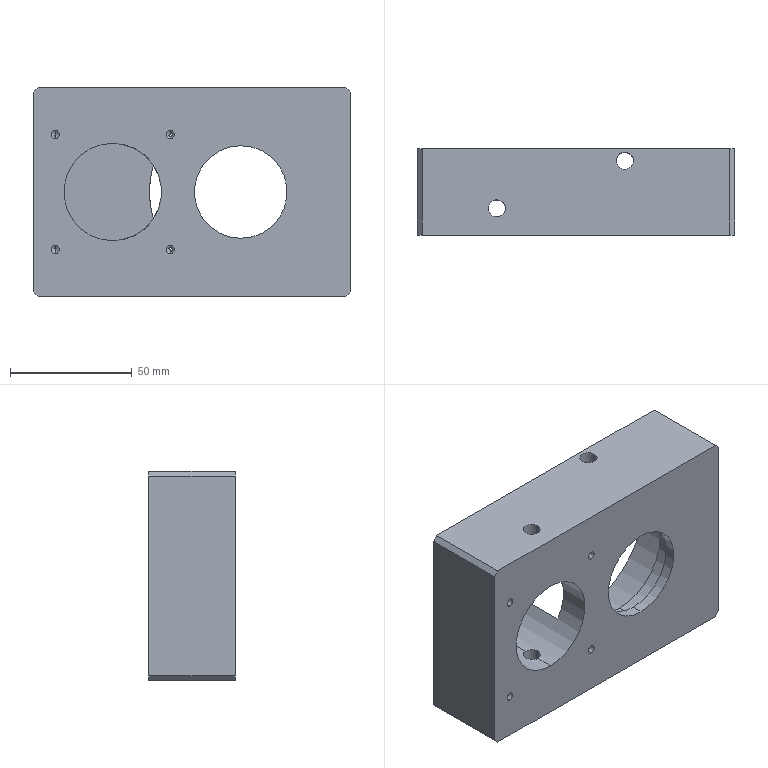Part | SolidWorks | features BaseBody 1 | 1 solid | 64 faces | box 130 x 35.485 x 86 mm | volume 236354 mm3 | cylinder 34 | cone 16 | plane 14 | commonest cylinder face diameters 3.3 x8 4.2 x8 7 x8 38 x2 40 x2 44 x2